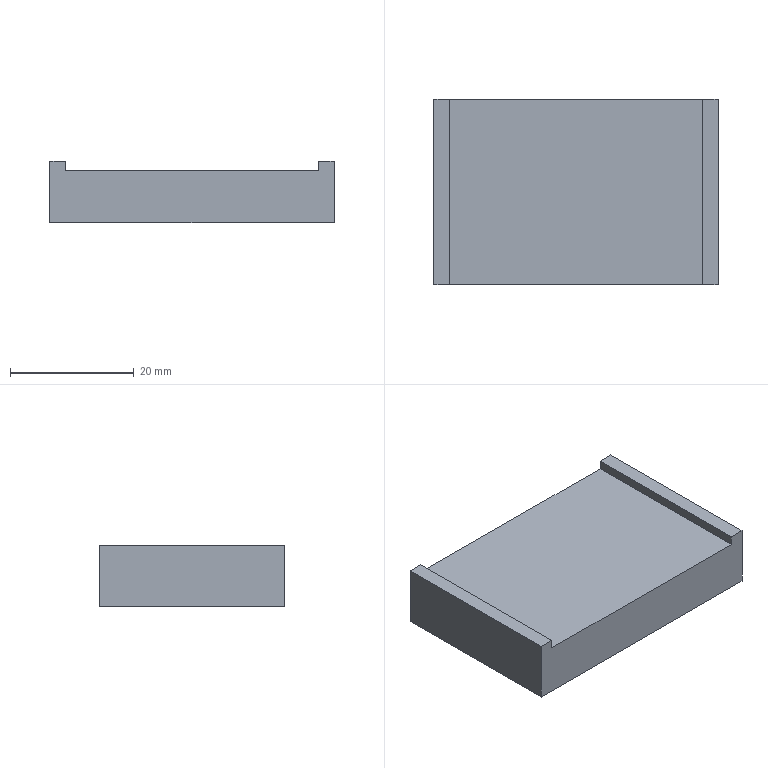Part | SolidWorks | features 3DProfileFeature 1, Extrusion 1, HoleWzd 1, ICE 1, MirrorPattern 1 | 1 solid | 22 faces | box 46 x 30 x 10 mm | volume 11809 mm3 | plane 10 | cone 8 | cylinder 4 | commonest cylinder face diameters 3.3 x4
STEP:
#1=CARTESIAN_POINT('',(-16.,14.625,2.85));
#2=VERTEX_POINT('',#1);
#3=CARTESIAN_POINT('',(-16.,14.625,6.15));
#4=VERTEX_POINT('',#3);
#5=CARTESIAN_POINT('',(-16.,14.625,4.5));
#6=DIRECTION('',(0.,1.,0.));
#7=DIRECTION('',(0.,0.,1.));
#8=AXIS2_PLACEMENT_3D('',#5,#6,#7);
#9=CIRCLE('',#8,1.65);
#10=EDGE_CURVE('',#2,#4,#9,.T.);
#11=ORIENTED_EDGE('',*,*,#10,.F.);
#12=CARTESIAN_POINT('',(-16.,15.,2.475));
#13=VERTEX_POINT('',#12);
#14=CARTESIAN_POINT('',(-16.,15.,2.475));
#15=DIRECTION('',(0.,0.7071,-0.7071));
#16=VECTOR('',#15,1000.);
#17=LINE('',#14,#16);
#18=EDGE_CURVE('',#2,#13,#17,.T.);
#19=ORIENTED_EDGE('',*,*,#18,.T.);
#20=CARTESIAN_POINT('',(-16.,15.,6.525));
#21=VERTEX_POINT('',#20);
#22=CARTESIAN_POINT('',(-16.,15.,4.5));
#23=DIRECTION('',(0.,1.,0.));
#24=DIRECTION('',(0.,0.,1.));
#25=AXIS2_PLACEMENT_3D('',#22,#23,#24);
#26=CIRCLE('',#25,2.025);
#27=EDGE_CURVE('',#13,#21,#26,.T.);
#28=ORIENTED_EDGE('',*,*,#27,.T.);
#29=CARTESIAN_POINT('',(-16.,15.,6.525));
#30=DIRECTION('',(0.,0.7071,0.7071));
#31=VECTOR('',#30,1000.);
#32=LINE('',#29,#31);
#33=EDGE_CURVE('',#4,#21,#32,.T.);
#34=ORIENTED_EDGE('',*,*,#33,.F.);
#35=EDGE_LOOP('',(#11,#19,#28,#34));
#36=FACE_OUTER_BOUND('',#35,.T.);
#37=CARTESIAN_POINT('',(-16.,15.,4.5));
#38=DIRECTION('',(0.,1.,0.));
#39=DIRECTION('',(0.,0.,1.));
#40=AXIS2_PLACEMENT_3D('',#37,#38,#39);
#41=CONICAL_SURFACE('',#40,2.025,0.7854);
#42=ADVANCED_FACE('',(#36),#41,.F.);
#43=CARTESIAN_POINT('',(-16.,6.9,2.85));
#44=VERTEX_POINT('',#43);
#45=CARTESIAN_POINT('',(-16.,6.9,6.15));
#46=VERTEX_POINT('',#45);
#47=CARTESIAN_POINT('',(-16.,6.9,4.5));
#48=DIRECTION('',(0.,1.,0.));
#49=DIRECTION('',(0.,0.,1.));
#50=AXIS2_PLACEMENT_3D('',#47,#48,#49);
#51=CIRCLE('',#50,1.65);
#52=EDGE_CURVE('',#44,#46,#51,.T.);
#53=ORIENTED_EDGE('',*,*,#52,.F.);
#54=CARTESIAN_POINT('',(-16.,15.,2.85));
#55=DIRECTION('',(0.,1.,0.));
#56=VECTOR('',#55,1000.);
#57=LINE('',#54,#56);
#58=EDGE_CURVE('',#44,#2,#57,.T.);
#59=ORIENTED_EDGE('',*,*,#58,.T.);
#60=ORIENTED_EDGE('',*,*,#10,.T.);
#61=CARTESIAN_POINT('',(-16.,15.,6.15));
#62=DIRECTION('',(0.,1.,0.));
#63=VECTOR('',#62,1000.);
#64=LINE('',#61,#63);
#65=EDGE_CURVE('',#46,#4,#64,.T.);
#66=ORIENTED_EDGE('',*,*,#65,.F.);
#67=EDGE_LOOP('',(#53,#59,#60,#66));
#68=FACE_OUTER_BOUND('',#67,.T.);
#69=CARTESIAN_POINT('',(-16.,15.,4.5));
#70=DIRECTION('',(0.,1.,0.));
#71=DIRECTION('',(0.,0.,1.));
#72=AXIS2_PLACEMENT_3D('',#69,#70,#71);
#73=CYLINDRICAL_SURFACE('',#72,1.65);
#74=ADVANCED_FACE('',(#68),#73,.F.);
#75=CARTESIAN_POINT('',(-16.,5.909,4.5));
#76=VERTEX_POINT('',#75);
#77=CARTESIAN_POINT('',(-16.,6.9,6.15));
#78=DIRECTION('',(0.,0.515,0.8572));
#79=VECTOR('',#78,1000.);
#80=LINE('',#77,#79);
#81=EDGE_CURVE('',#76,#46,#80,.T.);
#82=ORIENTED_EDGE('',*,*,#81,.F.);
#83=CARTESIAN_POINT('',(-16.,6.9,2.85));
#84=DIRECTION('',(0.,0.515,-0.8572));
#85=VECTOR('',#84,1000.);
#86=LINE('',#83,#85);
#87=EDGE_CURVE('',#76,#44,#86,.T.);
#88=ORIENTED_EDGE('',*,*,#87,.T.);
#89=ORIENTED_EDGE('',*,*,#52,.T.);
#90=EDGE_LOOP('',(#82,#88,#89));
#91=FACE_OUTER_BOUND('',#90,.T.);
#92=CARTESIAN_POINT('',(-16.,6.9,4.5));
#93=DIRECTION('',(0.,1.,0.));
#94=DIRECTION('',(0.,0.,1.));
#95=AXIS2_PLACEMENT_3D('',#92,#93,#94);
#96=CONICAL_SURFACE('',#95,1.65,1.03);
#97=ADVANCED_FACE('',(#91),#96,.F.);
#98=CARTESIAN_POINT('',(16.,14.625,2.85));
#99=VERTEX_POINT('',#98);
#100=CARTESIAN_POINT('',(16.,14.625,6.15));
#101=VERTEX_POINT('',#100);
#102=CARTESIAN_POINT('',(16.,14.625,4.5));
#103=DIRECTION('',(0.,1.,0.));
#104=DIRECTION('',(0.,0.,1.));
#105=AXIS2_PLACEMENT_3D('',#102,#103,#104);
#106=CIRCLE('',#105,1.65);
#107=EDGE_CURVE('',#99,#101,#106,.T.);
#108=ORIENTED_EDGE('',*,*,#107,.F.);
#109=CARTESIAN_POINT('',(16.,15.,2.475));
#110=VERTEX_POINT('',#109);
#111=CARTESIAN_POINT('',(16.,15.,2.475));
#112=DIRECTION('',(0.,0.7071,-0.7071));
#113=VECTOR('',#112,1000.);
#114=LINE('',#111,#113);
#115=EDGE_CURVE('',#99,#110,#114,.T.);
#116=ORIENTED_EDGE('',*,*,#115,.T.);
#117=CARTESIAN_POINT('',(16.,15.,6.525));
#118=VERTEX_POINT('',#117);
#119=CARTESIAN_POINT('',(16.,15.,4.5));
#120=DIRECTION('',(0.,1.,0.));
#121=DIRECTION('',(0.,0.,1.));
#122=AXIS2_PLACEMENT_3D('',#119,#120,#121);
#123=CIRCLE('',#122,2.025);
#124=EDGE_CURVE('',#110,#118,#123,.T.);
#125=ORIENTED_EDGE('',*,*,#124,.T.);
#126=CARTESIAN_POINT('',(16.,15.,6.525));
#127=DIRECTION('',(0.,0.7071,0.7071));
#128=VECTOR('',#127,1000.);
#129=LINE('',#126,#128);
#130=EDGE_CURVE('',#101,#118,#129,.T.);
#131=ORIENTED_EDGE('',*,*,#130,.F.);
#132=EDGE_LOOP('',(#108,#116,#125,#131));
#133=FACE_OUTER_BOUND('',#132,.T.);
#134=CARTESIAN_POINT('',(16.,15.,4.5));
#135=DIRECTION('',(0.,1.,0.));
#136=DIRECTION('',(0.,0.,1.));
#137=AXIS2_PLACEMENT_3D('',#134,#135,#136);
#138=CONICAL_SURFACE('',#137,2.025,0.7854);
#139=ADVANCED_FACE('',(#133),#138,.F.);
#140=CARTESIAN_POINT('',(16.,6.9,2.85));
#141=VERTEX_POINT('',#140);
#142=CARTESIAN_POINT('',(16.,6.9,6.15));
#143=VERTEX_POINT('',#142);
#144=CARTESIAN_POINT('',(16.,6.9,4.5));
#145=DIRECTION('',(0.,1.,0.));
#146=DIRECTION('',(0.,0.,1.));
#147=AXIS2_PLACEMENT_3D('',#144,#145,#146);
#148=CIRCLE('',#147,1.65);
#149=EDGE_CURVE('',#141,#143,#148,.T.);
#150=ORIENTED_EDGE('',*,*,#149,.F.);
#151=CARTESIAN_POINT('',(16.,15.,2.85));
#152=DIRECTION('',(0.,1.,0.));
#153=VECTOR('',#152,1000.);
#154=LINE('',#151,#153);
#155=EDGE_CURVE('',#141,#99,#154,.T.);
#156=ORIENTED_EDGE('',*,*,#155,.T.);
#157=ORIENTED_EDGE('',*,*,#107,.T.);
#158=CARTESIAN_POINT('',(16.,15.,6.15));
#159=DIRECTION('',(0.,1.,0.));
#160=VECTOR('',#159,1000.);
#161=LINE('',#158,#160);
#162=EDGE_CURVE('',#143,#101,#161,.T.);
#163=ORIENTED_EDGE('',*,*,#162,.F.);
#164=EDGE_LOOP('',(#150,#156,#157,#163));
#165=FACE_OUTER_BOUND('',#164,.T.);
#166=CARTESIAN_POINT('',(16.,15.,4.5));
#167=DIRECTION('',(0.,1.,0.));
#168=DIRECTION('',(0.,0.,1.));
#169=AXIS2_PLACEMENT_3D('',#166,#167,#168);
#170=CYLINDRICAL_SURFACE('',#169,1.65);
#171=ADVANCED_FACE('',(#165),#170,.F.);
#172=CARTESIAN_POINT('',(16.,5.909,4.5));
#173=VERTEX_POINT('',#172);
#174=CARTESIAN_POINT('',(16.,6.9,6.15));
#175=DIRECTION('',(0.,0.515,0.8572));
#176=VECTOR('',#175,1000.);
#177=LINE('',#174,#176);
#178=EDGE_CURVE('',#173,#143,#177,.T.);
#179=ORIENTED_EDGE('',*,*,#178,.F.);
#180=CARTESIAN_POINT('',(16.,6.9,2.85));
#181=DIRECTION('',(0.,0.515,-0.8572));
#182=VECTOR('',#181,1000.);
#183=LINE('',#180,#182);
#184=EDGE_CURVE('',#173,#141,#183,.T.);
#185=ORIENTED_EDGE('',*,*,#184,.T.);
#186=ORIENTED_EDGE('',*,*,#149,.T.);
#187=EDGE_LOOP('',(#179,#185,#186));
#188=FACE_OUTER_BOUND('',#187,.T.);
#189=CARTESIAN_POINT('',(16.,6.9,4.5));
#190=DIRECTION('',(0.,1.,0.));
#191=DIRECTION('',(0.,0.,1.));
#192=AXIS2_PLACEMENT_3D('',#189,#190,#191);
#193=CONICAL_SURFACE('',#192,1.65,1.03);
#194=ADVANCED_FACE('',(#188),#193,.F.);
#195=CARTESIAN_POINT('',(23.,15.,10.));
#196=VERTEX_POINT('',#195);
#197=CARTESIAN_POINT('',(20.5,15.,10.));
#198=VERTEX_POINT('',#197);
#199=CARTESIAN_POINT('',(-23.,15.,10.));
#200=DIRECTION('',(-1.,0.,0.));
#201=VECTOR('',#200,1000.);
#202=LINE('',#199,#201);
#203=EDGE_CURVE('',#196,#198,#202,.T.);
#204=ORIENTED_EDGE('',*,*,#203,.T.);
#205=CARTESIAN_POINT('',(20.5,-15.,10.));
#206=VERTEX_POINT('',#205);
#207=CARTESIAN_POINT('',(20.5,15.,10.));
#208=DIRECTION('',(0.,1.,0.));
#209=VECTOR('',#208,1000.);
#210=LINE('',#207,#209);
#211=EDGE_CURVE('',#206,#198,#210,.T.);
#212=ORIENTED_EDGE('',*,*,#211,.F.);
#213=CARTESIAN_POINT('',(23.,-15.,10.));
#214=VERTEX_POINT('',#213);
#215=CARTESIAN_POINT('',(-23.,-15.,10.));
#216=DIRECTION('',(1.,0.,0.));
#217=VECTOR('',#216,1000.);
#218=LINE('',#215,#217);
#219=EDGE_CURVE('',#206,#214,#218,.T.);
#220=ORIENTED_EDGE('',*,*,#219,.T.);
#221=CARTESIAN_POINT('',(23.,-15.,10.));
#222=DIRECTION('',(0.,1.,0.));
#223=VECTOR('',#222,1000.);
#224=LINE('',#221,#223);
#225=EDGE_CURVE('',#214,#196,#224,.T.);
#226=ORIENTED_EDGE('',*,*,#225,.T.);
#227=EDGE_LOOP('',(#204,#212,#220,#226));
#228=FACE_OUTER_BOUND('',#227,.T.);
#229=CARTESIAN_POINT('',(0.,0.,10.));
#230=DIRECTION('',(0.,0.,-1.));
#231=DIRECTION('',(-1.,0.,0.));
#232=AXIS2_PLACEMENT_3D('',#229,#230,#231);
#233=PLANE('',#232);
#234=ADVANCED_FACE('',(#228),#233,.F.);
#235=CARTESIAN_POINT('',(23.,-15.,0.));
#236=VERTEX_POINT('',#235);
#237=CARTESIAN_POINT('',(23.,15.,0.));
#238=VERTEX_POINT('',#237);
#239=CARTESIAN_POINT('',(23.,-15.,0.));
#240=DIRECTION('',(0.,1.,0.));
#241=VECTOR('',#240,1000.);
#242=LINE('',#239,#241);
#243=EDGE_CURVE('',#236,#238,#242,.T.);
#244=ORIENTED_EDGE('',*,*,#243,.T.);
#245=CARTESIAN_POINT('',(23.,15.,10.));
#246=DIRECTION('',(0.,0.,-1.));
#247=VECTOR('',#246,1000.);
#248=LINE('',#245,#247);
#249=EDGE_CURVE('',#196,#238,#248,.T.);
#250=ORIENTED_EDGE('',*,*,#249,.F.);
#251=ORIENTED_EDGE('',*,*,#225,.F.);
#252=CARTESIAN_POINT('',(23.,-15.,10.));
#253=DIRECTION('',(0.,0.,-1.));
#254=VECTOR('',#253,1000.);
#255=LINE('',#252,#254);
#256=EDGE_CURVE('',#214,#236,#255,.T.);
#257=ORIENTED_EDGE('',*,*,#256,.T.);
#258=EDGE_LOOP('',(#244,#250,#251,#257));
#259=FACE_OUTER_BOUND('',#258,.T.);
#260=CARTESIAN_POINT('',(23.,-15.,10.));
#261=DIRECTION('',(-1.,0.,0.));
#262=DIRECTION('',(0.,0.,1.));
#263=AXIS2_PLACEMENT_3D('',#260,#261,#262);
#264=PLANE('',#263);
#265=ADVANCED_FACE('',(#259),#264,.F.);
#266=CARTESIAN_POINT('',(-16.,15.,4.5));
#267=DIRECTION('',(0.,1.,0.));
#268=DIRECTION('',(0.,0.,1.));
#269=AXIS2_PLACEMENT_3D('',#266,#267,#268);
#270=CIRCLE('',#269,2.025);
#271=EDGE_CURVE('',#21,#13,#270,.T.);
#272=ORIENTED_EDGE('',*,*,#271,.F.);
#273=ORIENTED_EDGE('',*,*,#27,.F.);
#274=EDGE_LOOP('',(#272,#273));
#275=FACE_BOUND('',#274,.T.);
#276=CARTESIAN_POINT('',(16.,15.,4.5));
#277=DIRECTION('',(0.,1.,0.));
#278=DIRECTION('',(0.,0.,1.));
#279=AXIS2_PLACEMENT_3D('',#276,#277,#278);
#280=CIRCLE('',#279,2.025);
#281=EDGE_CURVE('',#118,#110,#280,.T.);
#282=ORIENTED_EDGE('',*,*,#281,.F.);
#283=ORIENTED_EDGE('',*,*,#124,.F.);
#284=EDGE_LOOP('',(#282,#283));
#285=FACE_BOUND('',#284,.T.);
#286=CARTESIAN_POINT('',(20.5,15.,8.5));
#287=VERTEX_POINT('',#286);
#288=CARTESIAN_POINT('',(-20.5,15.,8.5));
#289=VERTEX_POINT('',#288);
#290=CARTESIAN_POINT('',(-20.5,15.,8.5));
#291=DIRECTION('',(-1.,0.,0.));
#292=VECTOR('',#291,1000.);
#293=LINE('',#290,#292);
#294=EDGE_CURVE('',#287,#289,#293,.T.);
#295=ORIENTED_EDGE('',*,*,#294,.F.);
#296=CARTESIAN_POINT('',(20.5,15.,8.5));
#297=DIRECTION('',(0.,0.,1.));
#298=VECTOR('',#297,1000.);
#299=LINE('',#296,#298);
#300=EDGE_CURVE('',#287,#198,#299,.T.);
#301=ORIENTED_EDGE('',*,*,#300,.T.);
#302=ORIENTED_EDGE('',*,*,#203,.F.);
#303=ORIENTED_EDGE('',*,*,#249,.T.);
#304=CARTESIAN_POINT('',(-23.,15.,0.));
#305=VERTEX_POINT('',#304);
#306=CARTESIAN_POINT('',(-23.,15.,0.));
#307=DIRECTION('',(-1.,0.,0.));
#308=VECTOR('',#307,1000.);
#309=LINE('',#306,#308);
#310=EDGE_CURVE('',#238,#305,#309,.T.);
#311=ORIENTED_EDGE('',*,*,#310,.T.);
#312=CARTESIAN_POINT('',(-23.,15.,10.));
#313=VERTEX_POINT('',#312);
#314=CARTESIAN_POINT('',(-23.,15.,10.));
#315=DIRECTION('',(0.,0.,-1.));
#316=VECTOR('',#315,1000.);
#317=LINE('',#314,#316);
#318=EDGE_CURVE('',#313,#305,#317,.T.);
#319=ORIENTED_EDGE('',*,*,#318,.F.);
#320=CARTESIAN_POINT('',(-20.5,15.,10.));
#321=VERTEX_POINT('',#320);
#322=CARTESIAN_POINT('',(-23.,15.,10.));
#323=DIRECTION('',(-1.,0.,0.));
#324=VECTOR('',#323,1000.);
#325=LINE('',#322,#324);
#326=EDGE_CURVE('',#321,#313,#325,.T.);
#327=ORIENTED_EDGE('',*,*,#326,.F.);
#328=CARTESIAN_POINT('',(-20.5,15.,8.5));
#329=DIRECTION('',(0.,0.,1.));
#330=VECTOR('',#329,1000.);
#331=LINE('',#328,#330);
#332=EDGE_CURVE('',#289,#321,#331,.T.);
#333=ORIENTED_EDGE('',*,*,#332,.F.);
#334=EDGE_LOOP('',(#295,#301,#302,#303,#311,#319,#327,#333));
#335=FACE_OUTER_BOUND('',#334,.T.);
#336=CARTESIAN_POINT('',(-23.,15.,10.));
#337=DIRECTION('',(0.,-1.,0.));
#338=DIRECTION('',(0.,0.,-1.));
#339=AXIS2_PLACEMENT_3D('',#336,#337,#338);
#340=PLANE('',#339);
#341=ADVANCED_FACE('',(#275,#285,#335),#340,.F.);
#342=CARTESIAN_POINT('',(-23.,-15.,0.));
#343=VERTEX_POINT('',#342);
#344=CARTESIAN_POINT('',(-23.,-15.,0.));
#345=DIRECTION('',(0.,-1.,0.));
#346=VECTOR('',#345,1000.);
#347=LINE('',#344,#346);
#348=EDGE_CURVE('',#305,#343,#347,.T.);
#349=ORIENTED_EDGE('',*,*,#348,.T.);
#350=CARTESIAN_POINT('',(-23.,-15.,10.));
#351=VERTEX_POINT('',#350);
#352=CARTESIAN_POINT('',(-23.,-15.,10.));
#353=DIRECTION('',(0.,0.,-1.));
#354=VECTOR('',#353,1000.);
#355=LINE('',#352,#354);
#356=EDGE_CURVE('',#351,#343,#355,.T.);
#357=ORIENTED_EDGE('',*,*,#356,.F.);
#358=CARTESIAN_POINT('',(-23.,-15.,10.));
#359=DIRECTION('',(0.,-1.,0.));
#360=VECTOR('',#359,1000.);
#361=LINE('',#358,#360);
#362=EDGE_CURVE('',#313,#351,#361,.T.);
#363=ORIENTED_EDGE('',*,*,#362,.F.);
#364=ORIENTED_EDGE('',*,*,#318,.T.);
#365=EDGE_LOOP('',(#349,#357,#363,#364));
#366=FACE_OUTER_BOUND('',#365,.T.);
#367=CARTESIAN_POINT('',(-23.,-15.,10.));
#368=DIRECTION('',(1.,0.,0.));
#369=DIRECTION('',(0.,0.,-1.));
#370=AXIS2_PLACEMENT_3D('',#367,#368,#369);
#371=PLANE('',#370);
#372=ADVANCED_FACE('',(#366),#371,.F.);
#373=ORIENTED_EDGE('',*,*,#219,.F.);
#374=CARTESIAN_POINT('',(20.5,-15.,8.5));
#375=VERTEX_POINT('',#374);
#376=CARTESIAN_POINT('',(20.5,-15.,8.5));
#377=DIRECTION('',(0.,0.,1.));
#378=VECTOR('',#377,1000.);
#379=LINE('',#376,#378);
#380=EDGE_CURVE('',#375,#206,#379,.T.);
#381=ORIENTED_EDGE('',*,*,#380,.F.);
#382=CARTESIAN_POINT('',(-20.5,-15.,8.5));
#383=VERTEX_POINT('',#382);
#384=CARTESIAN_POINT('',(-20.5,-15.,8.5));
#385=DIRECTION('',(1.,0.,0.));
#386=VECTOR('',#385,1000.);
#387=LINE('',#384,#386);
#388=EDGE_CURVE('',#383,#375,#387,.T.);
#389=ORIENTED_EDGE('',*,*,#388,.F.);
#390=CARTESIAN_POINT('',(-20.5,-15.,10.));
#391=VERTEX_POINT('',#390);
#392=CARTESIAN_POINT('',(-20.5,-15.,8.5));
#393=DIRECTION('',(0.,0.,1.));
#394=VECTOR('',#393,1000.);
#395=LINE('',#392,#394);
#396=EDGE_CURVE('',#383,#391,#395,.T.);
#397=ORIENTED_EDGE('',*,*,#396,.T.);
#398=CARTESIAN_POINT('',(-23.,-15.,10.));
#399=DIRECTION('',(1.,0.,0.));
#400=VECTOR('',#399,1000.);
#401=LINE('',#398,#400);
#402=EDGE_CURVE('',#351,#391,#401,.T.);
#403=ORIENTED_EDGE('',*,*,#402,.F.);
#404=ORIENTED_EDGE('',*,*,#356,.T.);
#405=CARTESIAN_POINT('',(-23.,-15.,0.));
#406=DIRECTION('',(1.,0.,0.));
#407=VECTOR('',#406,1000.);
#408=LINE('',#405,#407);
#409=EDGE_CURVE('',#343,#236,#408,.T.);
#410=ORIENTED_EDGE('',*,*,#409,.T.);
#411=ORIENTED_EDGE('',*,*,#256,.F.);
#412=EDGE_LOOP('',(#373,#381,#389,#397,#403,#404,#410,#411));
#413=FACE_OUTER_BOUND('',#412,.T.);
#414=CARTESIAN_POINT('',(-23.,-15.,10.));
#415=DIRECTION('',(0.,1.,0.));
#416=DIRECTION('',(0.,0.,1.));
#417=AXIS2_PLACEMENT_3D('',#414,#415,#416);
#418=PLANE('',#417);
#419=ADVANCED_FACE('',(#413),#418,.F.);
#420=ORIENTED_EDGE('',*,*,#402,.T.);
#421=CARTESIAN_POINT('',(-20.5,15.,10.));
#422=DIRECTION('',(0.,-1.,0.));
#423=VECTOR('',#422,1000.);
#424=LINE('',#421,#423);
#425=EDGE_CURVE('',#321,#391,#424,.T.);
#426=ORIENTED_EDGE('',*,*,#425,.F.);
#427=ORIENTED_EDGE('',*,*,#326,.T.);
#428=ORIENTED_EDGE('',*,*,#362,.T.);
#429=EDGE_LOOP('',(#420,#426,#427,#428));
#430=FACE_OUTER_BOUND('',#429,.T.);
#431=CARTESIAN_POINT('',(0.,0.,10.));
#432=DIRECTION('',(0.,0.,-1.));
#433=DIRECTION('',(-1.,0.,0.));
#434=AXIS2_PLACEMENT_3D('',#431,#432,#433);
#435=PLANE('',#434);
#436=ADVANCED_FACE('',(#430),#435,.F.);
#437=ORIENTED_EDGE('',*,*,#243,.F.);
#438=ORIENTED_EDGE('',*,*,#409,.F.);
#439=ORIENTED_EDGE('',*,*,#348,.F.);
#440=ORIENTED_EDGE('',*,*,#310,.F.);
#441=EDGE_LOOP('',(#437,#438,#439,#440));
#442=FACE_OUTER_BOUND('',#441,.T.);
#443=CARTESIAN_POINT('',(0.,0.,0.));
#444=DIRECTION('',(0.,0.,-1.));
#445=DIRECTION('',(-1.,0.,0.));
#446=AXIS2_PLACEMENT_3D('',#443,#444,#445);
#447=PLANE('',#446);
#448=ADVANCED_FACE('',(#442),#447,.T.);
#449=ORIENTED_EDGE('',*,*,#211,.T.);
#450=ORIENTED_EDGE('',*,*,#300,.F.);
#451=CARTESIAN_POINT('',(20.5,15.,8.5));
#452=DIRECTION('',(0.,1.,0.));
#453=VECTOR('',#452,1000.);
#454=LINE('',#451,#453);
#455=EDGE_CURVE('',#375,#287,#454,.T.);
#456=ORIENTED_EDGE('',*,*,#455,.F.);
#457=ORIENTED_EDGE('',*,*,#380,.T.);
#458=EDGE_LOOP('',(#449,#450,#456,#457));
#459=FACE_OUTER_BOUND('',#458,.T.);
#460=CARTESIAN_POINT('',(20.5,15.,8.5));
#461=DIRECTION('',(1.,0.,0.));
#462=DIRECTION('',(0.,0.,-1.));
#463=AXIS2_PLACEMENT_3D('',#460,#461,#462);
#464=PLANE('',#463);
#465=ADVANCED_FACE('',(#459),#464,.F.);
#466=ORIENTED_EDGE('',*,*,#425,.T.);
#467=ORIENTED_EDGE('',*,*,#396,.F.);
#468=CARTESIAN_POINT('',(-20.5,15.,8.5));
#469=DIRECTION('',(0.,-1.,0.));
#470=VECTOR('',#469,1000.);
#471=LINE('',#468,#470);
#472=EDGE_CURVE('',#289,#383,#471,.T.);
#473=ORIENTED_EDGE('',*,*,#472,.F.);
#474=ORIENTED_EDGE('',*,*,#332,.T.);
#475=EDGE_LOOP('',(#466,#467,#473,#474));
#476=FACE_OUTER_BOUND('',#475,.T.);
#477=CARTESIAN_POINT('',(-20.5,15.,8.5));
#478=DIRECTION('',(-1.,0.,0.));
#479=DIRECTION('',(0.,0.,1.));
#480=AXIS2_PLACEMENT_3D('',#477,#478,#479);
#481=PLANE('',#480);
#482=ADVANCED_FACE('',(#476),#481,.F.);
#483=ORIENTED_EDGE('',*,*,#455,.T.);
#484=ORIENTED_EDGE('',*,*,#294,.T.);
#485=ORIENTED_EDGE('',*,*,#472,.T.);
#486=ORIENTED_EDGE('',*,*,#388,.T.);
#487=EDGE_LOOP('',(#483,#484,#485,#486));
#488=FACE_OUTER_BOUND('',#487,.T.);
#489=CARTESIAN_POINT('',(0.,0.,8.5));
#490=DIRECTION('',(0.,0.,1.));
#491=DIRECTION('',(1.,0.,0.));
#492=AXIS2_PLACEMENT_3D('',#489,#490,#491);
#493=PLANE('',#492);
#494=ADVANCED_FACE('',(#488),#493,.T.);
#495=ORIENTED_EDGE('',*,*,#184,.F.);
#496=ORIENTED_EDGE('',*,*,#178,.T.);
#497=CARTESIAN_POINT('',(16.,6.9,4.5));
#498=DIRECTION('',(0.,1.,0.));
#499=DIRECTION('',(0.,0.,1.));
#500=AXIS2_PLACEMENT_3D('',#497,#498,#499);
#501=CIRCLE('',#500,1.65);
#502=EDGE_CURVE('',#143,#141,#501,.T.);
#503=ORIENTED_EDGE('',*,*,#502,.T.);
#504=EDGE_LOOP('',(#495,#496,#503));
#505=FACE_OUTER_BOUND('',#504,.T.);
#506=CARTESIAN_POINT('',(16.,6.9,4.5));
#507=DIRECTION('',(0.,1.,0.));
#508=DIRECTION('',(0.,0.,1.));
#509=AXIS2_PLACEMENT_3D('',#506,#507,#508);
#510=CONICAL_SURFACE('',#509,1.65,1.03);
#511=ADVANCED_FACE('',(#505),#510,.F.);
#512=ORIENTED_EDGE('',*,*,#155,.F.);
#513=ORIENTED_EDGE('',*,*,#502,.F.);
#514=ORIENTED_EDGE('',*,*,#162,.T.);
#515=CARTESIAN_POINT('',(16.,14.625,4.5));
#516=DIRECTION('',(0.,1.,0.));
#517=DIRECTION('',(0.,0.,1.));
#518=AXIS2_PLACEMENT_3D('',#515,#516,#517);
#519=CIRCLE('',#518,1.65);
#520=EDGE_CURVE('',#101,#99,#519,.T.);
#521=ORIENTED_EDGE('',*,*,#520,.T.);
#522=EDGE_LOOP('',(#512,#513,#514,#521));
#523=FACE_OUTER_BOUND('',#522,.T.);
#524=CARTESIAN_POINT('',(16.,15.,4.5));
#525=DIRECTION('',(0.,1.,0.));
#526=DIRECTION('',(0.,0.,1.));
#527=AXIS2_PLACEMENT_3D('',#524,#525,#526);
#528=CYLINDRICAL_SURFACE('',#527,1.65);
#529=ADVANCED_FACE('',(#523),#528,.F.);
#530=ORIENTED_EDGE('',*,*,#115,.F.);
#531=ORIENTED_EDGE('',*,*,#520,.F.);
#532=ORIENTED_EDGE('',*,*,#130,.T.);
#533=ORIENTED_EDGE('',*,*,#281,.T.);
#534=EDGE_LOOP('',(#530,#531,#532,#533));
#535=FACE_OUTER_BOUND('',#534,.T.);
#536=CARTESIAN_POINT('',(16.,15.,4.5));
#537=DIRECTION('',(0.,1.,0.));
#538=DIRECTION('',(0.,0.,1.));
#539=AXIS2_PLACEMENT_3D('',#536,#537,#538);
#540=CONICAL_SURFACE('',#539,2.025,0.7854);
#541=ADVANCED_FACE('',(#535),#540,.F.);
#542=ORIENTED_EDGE('',*,*,#87,.F.);
#543=ORIENTED_EDGE('',*,*,#81,.T.);
#544=CARTESIAN_POINT('',(-16.,6.9,4.5));
#545=DIRECTION('',(0.,1.,0.));
#546=DIRECTION('',(0.,0.,1.));
#547=AXIS2_PLACEMENT_3D('',#544,#545,#546);
#548=CIRCLE('',#547,1.65);
#549=EDGE_CURVE('',#46,#44,#548,.T.);
#550=ORIENTED_EDGE('',*,*,#549,.T.);
#551=EDGE_LOOP('',(#542,#543,#550));
#552=FACE_OUTER_BOUND('',#551,.T.);
#553=CARTESIAN_POINT('',(-16.,6.9,4.5));
#554=DIRECTION('',(0.,1.,0.));
#555=DIRECTION('',(0.,0.,1.));
#556=AXIS2_PLACEMENT_3D('',#553,#554,#555);
#557=CONICAL_SURFACE('',#556,1.65,1.03);
#558=ADVANCED_FACE('',(#552),#557,.F.);
#559=ORIENTED_EDGE('',*,*,#58,.F.);
#560=ORIENTED_EDGE('',*,*,#549,.F.);
#561=ORIENTED_EDGE('',*,*,#65,.T.);
#562=CARTESIAN_POINT('',(-16.,14.625,4.5));
#563=DIRECTION('',(0.,1.,0.));
#564=DIRECTION('',(0.,0.,1.));
#565=AXIS2_PLACEMENT_3D('',#562,#563,#564);
#566=CIRCLE('',#565,1.65);
#567=EDGE_CURVE('',#4,#2,#566,.T.);
#568=ORIENTED_EDGE('',*,*,#567,.T.);
#569=EDGE_LOOP('',(#559,#560,#561,#568));
#570=FACE_OUTER_BOUND('',#569,.T.);
#571=CARTESIAN_POINT('',(-16.,15.,4.5));
#572=DIRECTION('',(0.,1.,0.));
#573=DIRECTION('',(0.,0.,1.));
#574=AXIS2_PLACEMENT_3D('',#571,#572,#573);
#575=CYLINDRICAL_SURFACE('',#574,1.65);
#576=ADVANCED_FACE('',(#570),#575,.F.);
#577=ORIENTED_EDGE('',*,*,#18,.F.);
#578=ORIENTED_EDGE('',*,*,#567,.F.);
#579=ORIENTED_EDGE('',*,*,#33,.T.);
#580=ORIENTED_EDGE('',*,*,#271,.T.);
#581=EDGE_LOOP('',(#577,#578,#579,#580));
#582=FACE_OUTER_BOUND('',#581,.T.);
#583=CARTESIAN_POINT('',(-16.,15.,4.5));
#584=DIRECTION('',(0.,1.,0.));
#585=DIRECTION('',(0.,0.,1.));
#586=AXIS2_PLACEMENT_3D('',#583,#584,#585);
#587=CONICAL_SURFACE('',#586,2.025,0.7854);
#588=ADVANCED_FACE('',(#582),#587,.F.);
#589=CLOSED_SHELL('',(#42,#74,#97,#139,#171,#194,#234,#265,#341,#372,#419,#436,#448,#465,#482,#494,#511,#529,#541,#558,#576,#588));
#590=MANIFOLD_SOLID_BREP('',#589);
#591=CARTESIAN_POINT('',(0.,0.,0.));
#592=DIRECTION('',(0.,0.,1.));
#593=DIRECTION('',(1.,0.,0.));
#594=AXIS2_PLACEMENT_3D('',#591,#592,#593);
#595=(LENGTH_UNIT()NAMED_UNIT(*)SI_UNIT(.MILLI.,.METRE.));
#596=UNCERTAINTY_MEASURE_WITH_UNIT(LENGTH_MEASURE(0.00001),#595,'','');
#597=(NAMED_UNIT(*)PLANE_ANGLE_UNIT()SI_UNIT($,.RADIAN.));
#598=(NAMED_UNIT(*)SI_UNIT($,.STERADIAN.)SOLID_ANGLE_UNIT());
#599=(GEOMETRIC_REPRESENTATION_CONTEXT(3)GLOBAL_UNCERTAINTY_ASSIGNED_CONTEXT((#596))GLOBAL_UNIT_ASSIGNED_CONTEXT((#595,#597,#598))REPRESENTATION_CONTEXT('',''));
#600=ADVANCED_BREP_SHAPE_REPRESENTATION('',(#590,#594),#599);